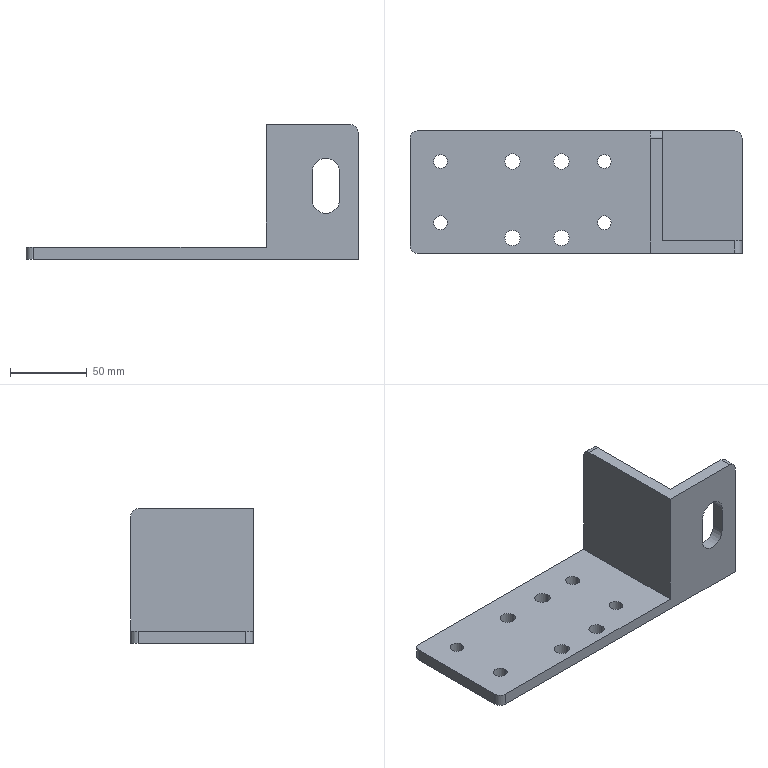Part | SolidWorks | features BaseBody 1 | 1 solid | 37 faces | box 217 x 80 x 88 mm | volume 213969 mm3 | cylinder 24 | plane 13 | commonest cylinder face diameters 10 x13 9 x8 18 x3
STEP:
#1=CARTESIAN_POINT('',(-84.,20.,8.));
#2=VERTEX_POINT('',#1);
#3=CARTESIAN_POINT('',(-93.,20.,8.));
#4=VERTEX_POINT('',#3);
#5=CARTESIAN_POINT('',(-88.5,20.,8.));
#6=DIRECTION('',(0.,0.,-1.));
#7=DIRECTION('',(-1.,0.,0.));
#8=AXIS2_PLACEMENT_3D('',#5,#6,#7);
#9=CIRCLE('',#8,4.5);
#10=EDGE_CURVE('',#2,#4,#9,.T.);
#11=ORIENTED_EDGE('',*,*,#10,.F.);
#12=CARTESIAN_POINT('',(-84.,20.,0.));
#13=VERTEX_POINT('',#12);
#14=CARTESIAN_POINT('',(-84.,20.,10.));
#15=DIRECTION('',(0.,0.,-1.));
#16=VECTOR('',#15,1000.);
#17=LINE('',#14,#16);
#18=EDGE_CURVE('',#2,#13,#17,.T.);
#19=ORIENTED_EDGE('',*,*,#18,.T.);
#20=CARTESIAN_POINT('',(-93.,20.,0.));
#21=VERTEX_POINT('',#20);
#22=CARTESIAN_POINT('',(-88.5,20.,0.));
#23=DIRECTION('',(0.,0.,-1.));
#24=DIRECTION('',(-1.,0.,0.));
#25=AXIS2_PLACEMENT_3D('',#22,#23,#24);
#26=CIRCLE('',#25,4.5);
#27=EDGE_CURVE('',#13,#21,#26,.T.);
#28=ORIENTED_EDGE('',*,*,#27,.T.);
#29=CARTESIAN_POINT('',(-93.,20.,10.));
#30=DIRECTION('',(0.,0.,-1.));
#31=VECTOR('',#30,1000.);
#32=LINE('',#29,#31);
#33=EDGE_CURVE('',#4,#21,#32,.T.);
#34=ORIENTED_EDGE('',*,*,#33,.F.);
#35=EDGE_LOOP('',(#11,#19,#28,#34));
#36=FACE_OUTER_BOUND('',#35,.T.);
#37=CARTESIAN_POINT('',(-88.5,20.,10.));
#38=DIRECTION('',(0.,0.,-1.));
#39=DIRECTION('',(-1.,0.,0.));
#40=AXIS2_PLACEMENT_3D('',#37,#38,#39);
#41=CYLINDRICAL_SURFACE('',#40,4.5);
#42=ADVANCED_FACE('',(#36),#41,.F.);
#43=CARTESIAN_POINT('',(23.,-20.,8.));
#44=VERTEX_POINT('',#43);
#45=CARTESIAN_POINT('',(14.,-20.,8.));
#46=VERTEX_POINT('',#45);
#47=CARTESIAN_POINT('',(18.5,-20.,8.));
#48=DIRECTION('',(0.,0.,-1.));
#49=DIRECTION('',(-1.,0.,0.));
#50=AXIS2_PLACEMENT_3D('',#47,#48,#49);
#51=CIRCLE('',#50,4.5);
#52=EDGE_CURVE('',#44,#46,#51,.T.);
#53=ORIENTED_EDGE('',*,*,#52,.F.);
#54=CARTESIAN_POINT('',(23.,-20.,0.));
#55=VERTEX_POINT('',#54);
#56=CARTESIAN_POINT('',(23.,-20.,10.));
#57=DIRECTION('',(0.,0.,-1.));
#58=VECTOR('',#57,1000.);
#59=LINE('',#56,#58);
#60=EDGE_CURVE('',#44,#55,#59,.T.);
#61=ORIENTED_EDGE('',*,*,#60,.T.);
#62=CARTESIAN_POINT('',(14.,-20.,0.));
#63=VERTEX_POINT('',#62);
#64=CARTESIAN_POINT('',(18.5,-20.,0.));
#65=DIRECTION('',(0.,0.,-1.));
#66=DIRECTION('',(-1.,0.,0.));
#67=AXIS2_PLACEMENT_3D('',#64,#65,#66);
#68=CIRCLE('',#67,4.5);
#69=EDGE_CURVE('',#55,#63,#68,.T.);
#70=ORIENTED_EDGE('',*,*,#69,.T.);
#71=CARTESIAN_POINT('',(14.,-20.,10.));
#72=DIRECTION('',(0.,0.,-1.));
#73=VECTOR('',#72,1000.);
#74=LINE('',#71,#73);
#75=EDGE_CURVE('',#46,#63,#74,.T.);
#76=ORIENTED_EDGE('',*,*,#75,.F.);
#77=EDGE_LOOP('',(#53,#61,#70,#76));
#78=FACE_OUTER_BOUND('',#77,.T.);
#79=CARTESIAN_POINT('',(18.5,-20.,10.));
#80=DIRECTION('',(0.,0.,-1.));
#81=DIRECTION('',(-1.,0.,0.));
#82=AXIS2_PLACEMENT_3D('',#79,#80,#81);
#83=CYLINDRICAL_SURFACE('',#82,4.5);
#84=ADVANCED_FACE('',(#78),#83,.F.);
#85=CARTESIAN_POINT('',(23.,20.,8.));
#86=VERTEX_POINT('',#85);
#87=CARTESIAN_POINT('',(14.,20.,8.));
#88=VERTEX_POINT('',#87);
#89=CARTESIAN_POINT('',(18.5,20.,8.));
#90=DIRECTION('',(0.,0.,-1.));
#91=DIRECTION('',(-1.,0.,0.));
#92=AXIS2_PLACEMENT_3D('',#89,#90,#91);
#93=CIRCLE('',#92,4.5);
#94=EDGE_CURVE('',#86,#88,#93,.T.);
#95=ORIENTED_EDGE('',*,*,#94,.F.);
#96=CARTESIAN_POINT('',(23.,20.,0.));
#97=VERTEX_POINT('',#96);
#98=CARTESIAN_POINT('',(23.,20.,10.));
#99=DIRECTION('',(0.,0.,-1.));
#100=VECTOR('',#99,1000.);
#101=LINE('',#98,#100);
#102=EDGE_CURVE('',#86,#97,#101,.T.);
#103=ORIENTED_EDGE('',*,*,#102,.T.);
#104=CARTESIAN_POINT('',(14.,20.,0.));
#105=VERTEX_POINT('',#104);
#106=CARTESIAN_POINT('',(18.5,20.,0.));
#107=DIRECTION('',(0.,0.,-1.));
#108=DIRECTION('',(-1.,0.,0.));
#109=AXIS2_PLACEMENT_3D('',#106,#107,#108);
#110=CIRCLE('',#109,4.5);
#111=EDGE_CURVE('',#97,#105,#110,.T.);
#112=ORIENTED_EDGE('',*,*,#111,.T.);
#113=CARTESIAN_POINT('',(14.,20.,10.));
#114=DIRECTION('',(0.,0.,-1.));
#115=VECTOR('',#114,1000.);
#116=LINE('',#113,#115);
#117=EDGE_CURVE('',#88,#105,#116,.T.);
#118=ORIENTED_EDGE('',*,*,#117,.F.);
#119=EDGE_LOOP('',(#95,#103,#112,#118));
#120=FACE_OUTER_BOUND('',#119,.T.);
#121=CARTESIAN_POINT('',(18.5,20.,10.));
#122=DIRECTION('',(0.,0.,-1.));
#123=DIRECTION('',(-1.,0.,0.));
#124=AXIS2_PLACEMENT_3D('',#121,#122,#123);
#125=CYLINDRICAL_SURFACE('',#124,4.5);
#126=ADVANCED_FACE('',(#120),#125,.F.);
#127=CARTESIAN_POINT('',(-84.,-20.,8.));
#128=VERTEX_POINT('',#127);
#129=CARTESIAN_POINT('',(-93.,-20.,8.));
#130=VERTEX_POINT('',#129);
#131=CARTESIAN_POINT('',(-88.5,-20.,8.));
#132=DIRECTION('',(0.,0.,-1.));
#133=DIRECTION('',(-1.,0.,0.));
#134=AXIS2_PLACEMENT_3D('',#131,#132,#133);
#135=CIRCLE('',#134,4.5);
#136=EDGE_CURVE('',#128,#130,#135,.T.);
#137=ORIENTED_EDGE('',*,*,#136,.F.);
#138=CARTESIAN_POINT('',(-84.,-20.,0.));
#139=VERTEX_POINT('',#138);
#140=CARTESIAN_POINT('',(-84.,-20.,10.));
#141=DIRECTION('',(0.,0.,-1.));
#142=VECTOR('',#141,1000.);
#143=LINE('',#140,#142);
#144=EDGE_CURVE('',#128,#139,#143,.T.);
#145=ORIENTED_EDGE('',*,*,#144,.T.);
#146=CARTESIAN_POINT('',(-93.,-20.,0.));
#147=VERTEX_POINT('',#146);
#148=CARTESIAN_POINT('',(-88.5,-20.,0.));
#149=DIRECTION('',(0.,0.,-1.));
#150=DIRECTION('',(-1.,0.,0.));
#151=AXIS2_PLACEMENT_3D('',#148,#149,#150);
#152=CIRCLE('',#151,4.5);
#153=EDGE_CURVE('',#139,#147,#152,.T.);
#154=ORIENTED_EDGE('',*,*,#153,.T.);
#155=CARTESIAN_POINT('',(-93.,-20.,10.));
#156=DIRECTION('',(0.,0.,-1.));
#157=VECTOR('',#156,1000.);
#158=LINE('',#155,#157);
#159=EDGE_CURVE('',#130,#147,#158,.T.);
#160=ORIENTED_EDGE('',*,*,#159,.F.);
#161=EDGE_LOOP('',(#137,#145,#154,#160));
#162=FACE_OUTER_BOUND('',#161,.T.);
#163=CARTESIAN_POINT('',(-88.5,-20.,10.));
#164=DIRECTION('',(0.,0.,-1.));
#165=DIRECTION('',(-1.,0.,0.));
#166=AXIS2_PLACEMENT_3D('',#163,#164,#165);
#167=CYLINDRICAL_SURFACE('',#166,4.5);
#168=ADVANCED_FACE('',(#162),#167,.F.);
#169=CARTESIAN_POINT('',(87.5,-40.,66.));
#170=VERTEX_POINT('',#169);
#171=CARTESIAN_POINT('',(96.5,-40.,57.));
#172=VERTEX_POINT('',#171);
#173=CARTESIAN_POINT('',(87.5,-40.,57.));
#174=DIRECTION('',(0.,1.,0.));
#175=DIRECTION('',(0.,0.,1.));
#176=AXIS2_PLACEMENT_3D('',#173,#174,#175);
#177=CIRCLE('',#176,9.);
#178=EDGE_CURVE('',#170,#172,#177,.T.);
#179=ORIENTED_EDGE('',*,*,#178,.F.);
#180=CARTESIAN_POINT('',(87.5,-32.,66.));
#181=VERTEX_POINT('',#180);
#182=CARTESIAN_POINT('',(87.5,-142.,66.));
#183=DIRECTION('',(0.,1.,0.));
#184=VECTOR('',#183,1000.);
#185=LINE('',#182,#184);
#186=EDGE_CURVE('',#170,#181,#185,.T.);
#187=ORIENTED_EDGE('',*,*,#186,.T.);
#188=CARTESIAN_POINT('',(96.5,-32.,57.));
#189=VERTEX_POINT('',#188);
#190=CARTESIAN_POINT('',(87.5,-32.,57.));
#191=DIRECTION('',(0.,1.,0.));
#192=DIRECTION('',(0.,0.,1.));
#193=AXIS2_PLACEMENT_3D('',#190,#191,#192);
#194=CIRCLE('',#193,9.);
#195=EDGE_CURVE('',#181,#189,#194,.T.);
#196=ORIENTED_EDGE('',*,*,#195,.T.);
#197=CARTESIAN_POINT('',(96.5,-142.,57.));
#198=DIRECTION('',(0.,1.,0.));
#199=VECTOR('',#198,1000.);
#200=LINE('',#197,#199);
#201=EDGE_CURVE('',#172,#189,#200,.T.);
#202=ORIENTED_EDGE('',*,*,#201,.F.);
#203=EDGE_LOOP('',(#179,#187,#196,#202));
#204=FACE_OUTER_BOUND('',#203,.T.);
#205=CARTESIAN_POINT('',(87.5,-142.,57.));
#206=DIRECTION('',(0.,1.,0.));
#207=DIRECTION('',(0.,0.,1.));
#208=AXIS2_PLACEMENT_3D('',#205,#206,#207);
#209=CYLINDRICAL_SURFACE('',#208,9.);
#210=ADVANCED_FACE('',(#204),#209,.F.);
#211=CARTESIAN_POINT('',(-4.5,20.,0.));
#212=VERTEX_POINT('',#211);
#213=CARTESIAN_POINT('',(-14.5,20.,0.));
#214=VERTEX_POINT('',#213);
#215=CARTESIAN_POINT('',(-9.5,20.,0.));
#216=DIRECTION('',(0.,0.,-1.));
#217=DIRECTION('',(-1.,0.,0.));
#218=AXIS2_PLACEMENT_3D('',#215,#216,#217);
#219=CIRCLE('',#218,5.);
#220=EDGE_CURVE('',#212,#214,#219,.T.);
#221=ORIENTED_EDGE('',*,*,#220,.T.);
#222=CARTESIAN_POINT('',(-14.5,20.,8.));
#223=VERTEX_POINT('',#222);
#224=CARTESIAN_POINT('',(-14.5,20.,-2.));
#225=DIRECTION('',(0.,0.,1.));
#226=VECTOR('',#225,1000.);
#227=LINE('',#224,#226);
#228=EDGE_CURVE('',#214,#223,#227,.T.);
#229=ORIENTED_EDGE('',*,*,#228,.T.);
#230=CARTESIAN_POINT('',(-4.5,20.,8.));
#231=VERTEX_POINT('',#230);
#232=CARTESIAN_POINT('',(-9.5,20.,8.));
#233=DIRECTION('',(0.,0.,1.));
#234=DIRECTION('',(1.,0.,0.));
#235=AXIS2_PLACEMENT_3D('',#232,#233,#234);
#236=CIRCLE('',#235,5.);
#237=EDGE_CURVE('',#223,#231,#236,.T.);
#238=ORIENTED_EDGE('',*,*,#237,.T.);
#239=CARTESIAN_POINT('',(-4.5,20.,-2.));
#240=DIRECTION('',(0.,0.,1.));
#241=VECTOR('',#240,1000.);
#242=LINE('',#239,#241);
#243=EDGE_CURVE('',#212,#231,#242,.T.);
#244=ORIENTED_EDGE('',*,*,#243,.F.);
#245=EDGE_LOOP('',(#221,#229,#238,#244));
#246=FACE_OUTER_BOUND('',#245,.T.);
#247=CARTESIAN_POINT('',(-9.5,20.,-2.));
#248=DIRECTION('',(0.,0.,1.));
#249=DIRECTION('',(1.,0.,0.));
#250=AXIS2_PLACEMENT_3D('',#247,#248,#249);
#251=CYLINDRICAL_SURFACE('',#250,5.);
#252=ADVANCED_FACE('',(#246),#251,.F.);
#253=CARTESIAN_POINT('',(-36.5,-30.,0.));
#254=VERTEX_POINT('',#253);
#255=CARTESIAN_POINT('',(-46.5,-30.,0.));
#256=VERTEX_POINT('',#255);
#257=CARTESIAN_POINT('',(-41.5,-30.,0.));
#258=DIRECTION('',(0.,0.,-1.));
#259=DIRECTION('',(-1.,0.,0.));
#260=AXIS2_PLACEMENT_3D('',#257,#258,#259);
#261=CIRCLE('',#260,5.);
#262=EDGE_CURVE('',#254,#256,#261,.T.);
#263=ORIENTED_EDGE('',*,*,#262,.T.);
#264=CARTESIAN_POINT('',(-46.5,-30.,8.));
#265=VERTEX_POINT('',#264);
#266=CARTESIAN_POINT('',(-46.5,-30.,-2.));
#267=DIRECTION('',(0.,0.,1.));
#268=VECTOR('',#267,1000.);
#269=LINE('',#266,#268);
#270=EDGE_CURVE('',#256,#265,#269,.T.);
#271=ORIENTED_EDGE('',*,*,#270,.T.);
#272=CARTESIAN_POINT('',(-36.5,-30.,8.));
#273=VERTEX_POINT('',#272);
#274=CARTESIAN_POINT('',(-41.5,-30.,8.));
#275=DIRECTION('',(0.,0.,1.));
#276=DIRECTION('',(1.,0.,0.));
#277=AXIS2_PLACEMENT_3D('',#274,#275,#276);
#278=CIRCLE('',#277,5.);
#279=EDGE_CURVE('',#265,#273,#278,.T.);
#280=ORIENTED_EDGE('',*,*,#279,.T.);
#281=CARTESIAN_POINT('',(-36.5,-30.,-2.));
#282=DIRECTION('',(0.,0.,1.));
#283=VECTOR('',#282,1000.);
#284=LINE('',#281,#283);
#285=EDGE_CURVE('',#254,#273,#284,.T.);
#286=ORIENTED_EDGE('',*,*,#285,.F.);
#287=EDGE_LOOP('',(#263,#271,#280,#286));
#288=FACE_OUTER_BOUND('',#287,.T.);
#289=CARTESIAN_POINT('',(-41.5,-30.,-2.));
#290=DIRECTION('',(0.,0.,1.));
#291=DIRECTION('',(1.,0.,0.));
#292=AXIS2_PLACEMENT_3D('',#289,#290,#291);
#293=CYLINDRICAL_SURFACE('',#292,5.);
#294=ADVANCED_FACE('',(#288),#293,.F.);
#295=CARTESIAN_POINT('',(-36.5,20.,0.));
#296=VERTEX_POINT('',#295);
#297=CARTESIAN_POINT('',(-46.5,20.,0.));
#298=VERTEX_POINT('',#297);
#299=CARTESIAN_POINT('',(-41.5,20.,0.));
#300=DIRECTION('',(0.,0.,-1.));
#301=DIRECTION('',(-1.,0.,0.));
#302=AXIS2_PLACEMENT_3D('',#299,#300,#301);
#303=CIRCLE('',#302,5.);
#304=EDGE_CURVE('',#296,#298,#303,.T.);
#305=ORIENTED_EDGE('',*,*,#304,.T.);
#306=CARTESIAN_POINT('',(-46.5,20.,8.));
#307=VERTEX_POINT('',#306);
#308=CARTESIAN_POINT('',(-46.5,20.,-2.));
#309=DIRECTION('',(0.,0.,1.));
#310=VECTOR('',#309,1000.);
#311=LINE('',#308,#310);
#312=EDGE_CURVE('',#298,#307,#311,.T.);
#313=ORIENTED_EDGE('',*,*,#312,.T.);
#314=CARTESIAN_POINT('',(-36.5,20.,8.));
#315=VERTEX_POINT('',#314);
#316=CARTESIAN_POINT('',(-41.5,20.,8.));
#317=DIRECTION('',(0.,0.,1.));
#318=DIRECTION('',(1.,0.,0.));
#319=AXIS2_PLACEMENT_3D('',#316,#317,#318);
#320=CIRCLE('',#319,5.);
#321=EDGE_CURVE('',#307,#315,#320,.T.);
#322=ORIENTED_EDGE('',*,*,#321,.T.);
#323=CARTESIAN_POINT('',(-36.5,20.,-2.));
#324=DIRECTION('',(0.,0.,1.));
#325=VECTOR('',#324,1000.);
#326=LINE('',#323,#325);
#327=EDGE_CURVE('',#296,#315,#326,.T.);
#328=ORIENTED_EDGE('',*,*,#327,.F.);
#329=EDGE_LOOP('',(#305,#313,#322,#328));
#330=FACE_OUTER_BOUND('',#329,.T.);
#331=CARTESIAN_POINT('',(-41.5,20.,-2.));
#332=DIRECTION('',(0.,0.,1.));
#333=DIRECTION('',(1.,0.,0.));
#334=AXIS2_PLACEMENT_3D('',#331,#332,#333);
#335=CYLINDRICAL_SURFACE('',#334,5.);
#336=ADVANCED_FACE('',(#330),#335,.F.);
#337=CARTESIAN_POINT('',(-4.5,-30.,0.));
#338=VERTEX_POINT('',#337);
#339=CARTESIAN_POINT('',(-14.5,-30.,0.));
#340=VERTEX_POINT('',#339);
#341=CARTESIAN_POINT('',(-9.5,-30.,0.));
#342=DIRECTION('',(0.,0.,-1.));
#343=DIRECTION('',(-1.,0.,0.));
#344=AXIS2_PLACEMENT_3D('',#341,#342,#343);
#345=CIRCLE('',#344,5.);
#346=EDGE_CURVE('',#338,#340,#345,.T.);
#347=ORIENTED_EDGE('',*,*,#346,.T.);
#348=CARTESIAN_POINT('',(-14.5,-30.,8.));
#349=VERTEX_POINT('',#348);
#350=CARTESIAN_POINT('',(-14.5,-30.,-2.));
#351=DIRECTION('',(0.,0.,1.));
#352=VECTOR('',#351,1000.);
#353=LINE('',#350,#352);
#354=EDGE_CURVE('',#340,#349,#353,.T.);
#355=ORIENTED_EDGE('',*,*,#354,.T.);
#356=CARTESIAN_POINT('',(-4.5,-30.,8.));
#357=VERTEX_POINT('',#356);
#358=CARTESIAN_POINT('',(-9.5,-30.,8.));
#359=DIRECTION('',(0.,0.,1.));
#360=DIRECTION('',(1.,0.,0.));
#361=AXIS2_PLACEMENT_3D('',#358,#359,#360);
#362=CIRCLE('',#361,5.);
#363=EDGE_CURVE('',#349,#357,#362,.T.);
#364=ORIENTED_EDGE('',*,*,#363,.T.);
#365=CARTESIAN_POINT('',(-4.5,-30.,-2.));
#366=DIRECTION('',(0.,0.,1.));
#367=VECTOR('',#366,1000.);
#368=LINE('',#365,#367);
#369=EDGE_CURVE('',#338,#357,#368,.T.);
#370=ORIENTED_EDGE('',*,*,#369,.F.);
#371=EDGE_LOOP('',(#347,#355,#364,#370));
#372=FACE_OUTER_BOUND('',#371,.T.);
#373=CARTESIAN_POINT('',(-9.5,-30.,-2.));
#374=DIRECTION('',(0.,0.,1.));
#375=DIRECTION('',(1.,0.,0.));
#376=AXIS2_PLACEMENT_3D('',#373,#374,#375);
#377=CYLINDRICAL_SURFACE('',#376,5.);
#378=ADVANCED_FACE('',(#372),#377,.F.);
#379=CARTESIAN_POINT('',(-88.5,20.,8.));
#380=DIRECTION('',(0.,0.,-1.));
#381=DIRECTION('',(-1.,0.,0.));
#382=AXIS2_PLACEMENT_3D('',#379,#380,#381);
#383=CIRCLE('',#382,4.5);
#384=EDGE_CURVE('',#4,#2,#383,.T.);
#385=ORIENTED_EDGE('',*,*,#384,.T.);
#386=ORIENTED_EDGE('',*,*,#10,.T.);
#387=EDGE_LOOP('',(#385,#386));
#388=FACE_BOUND('',#387,.T.);
#389=CARTESIAN_POINT('',(18.5,-20.,8.));
#390=DIRECTION('',(0.,0.,-1.));
#391=DIRECTION('',(-1.,0.,0.));
#392=AXIS2_PLACEMENT_3D('',#389,#390,#391);
#393=CIRCLE('',#392,4.5);
#394=EDGE_CURVE('',#46,#44,#393,.T.);
#395=ORIENTED_EDGE('',*,*,#394,.T.);
#396=ORIENTED_EDGE('',*,*,#52,.T.);
#397=EDGE_LOOP('',(#395,#396));
#398=FACE_BOUND('',#397,.T.);
#399=CARTESIAN_POINT('',(18.5,20.,8.));
#400=DIRECTION('',(0.,0.,-1.));
#401=DIRECTION('',(-1.,0.,0.));
#402=AXIS2_PLACEMENT_3D('',#399,#400,#401);
#403=CIRCLE('',#402,4.5);
#404=EDGE_CURVE('',#88,#86,#403,.T.);
#405=ORIENTED_EDGE('',*,*,#404,.T.);
#406=ORIENTED_EDGE('',*,*,#94,.T.);
#407=EDGE_LOOP('',(#405,#406));
#408=FACE_BOUND('',#407,.T.);
#409=CARTESIAN_POINT('',(-88.5,-20.,8.));
#410=DIRECTION('',(0.,0.,-1.));
#411=DIRECTION('',(-1.,0.,0.));
#412=AXIS2_PLACEMENT_3D('',#409,#410,#411);
#413=CIRCLE('',#412,4.5);
#414=EDGE_CURVE('',#130,#128,#413,.T.);
#415=ORIENTED_EDGE('',*,*,#414,.T.);
#416=ORIENTED_EDGE('',*,*,#136,.T.);
#417=EDGE_LOOP('',(#415,#416));
#418=FACE_BOUND('',#417,.T.);
#419=CARTESIAN_POINT('',(-9.5,-30.,8.));
#420=DIRECTION('',(0.,0.,1.));
#421=DIRECTION('',(1.,0.,0.));
#422=AXIS2_PLACEMENT_3D('',#419,#420,#421);
#423=CIRCLE('',#422,5.);
#424=EDGE_CURVE('',#357,#349,#423,.T.);
#425=ORIENTED_EDGE('',*,*,#424,.F.);
#426=ORIENTED_EDGE('',*,*,#363,.F.);
#427=EDGE_LOOP('',(#425,#426));
#428=FACE_BOUND('',#427,.T.);
#429=CARTESIAN_POINT('',(-41.5,20.,8.));
#430=DIRECTION('',(0.,0.,1.));
#431=DIRECTION('',(1.,0.,0.));
#432=AXIS2_PLACEMENT_3D('',#429,#430,#431);
#433=CIRCLE('',#432,5.);
#434=EDGE_CURVE('',#315,#307,#433,.T.);
#435=ORIENTED_EDGE('',*,*,#434,.F.);
#436=ORIENTED_EDGE('',*,*,#321,.F.);
#437=EDGE_LOOP('',(#435,#436));
#438=FACE_BOUND('',#437,.T.);
#439=CARTESIAN_POINT('',(-41.5,-30.,8.));
#440=DIRECTION('',(0.,0.,1.));
#441=DIRECTION('',(1.,0.,0.));
#442=AXIS2_PLACEMENT_3D('',#439,#440,#441);
#443=CIRCLE('',#442,5.);
#444=EDGE_CURVE('',#273,#265,#443,.T.);
#445=ORIENTED_EDGE('',*,*,#444,.F.);
#446=ORIENTED_EDGE('',*,*,#279,.F.);
#447=EDGE_LOOP('',(#445,#446));
#448=FACE_BOUND('',#447,.T.);
#449=CARTESIAN_POINT('',(-9.5,20.,8.));
#450=DIRECTION('',(0.,0.,1.));
#451=DIRECTION('',(1.,0.,0.));
#452=AXIS2_PLACEMENT_3D('',#449,#450,#451);
#453=CIRCLE('',#452,5.);
#454=EDGE_CURVE('',#231,#223,#453,.T.);
#455=ORIENTED_EDGE('',*,*,#454,.F.);
#456=ORIENTED_EDGE('',*,*,#237,.F.);
#457=EDGE_LOOP('',(#455,#456));
#458=FACE_BOUND('',#457,.T.);
#459=CARTESIAN_POINT('',(-108.5,35.,8.));
#460=VERTEX_POINT('',#459);
#461=CARTESIAN_POINT('',(-108.5,-35.,8.));
#462=VERTEX_POINT('',#461);
#463=CARTESIAN_POINT('',(-108.5,-40.,8.));
#464=DIRECTION('',(0.,-1.,0.));
#465=VECTOR('',#464,1000.);
#466=LINE('',#463,#465);
#467=EDGE_CURVE('',#460,#462,#466,.T.);
#468=ORIENTED_EDGE('',*,*,#467,.T.);
#469=CARTESIAN_POINT('',(-103.5,-40.,8.));
#470=VERTEX_POINT('',#469);
#471=CARTESIAN_POINT('',(-103.5,-35.,8.));
#472=DIRECTION('',(0.,0.,1.));
#473=DIRECTION('',(-1.,0.,0.));
#474=AXIS2_PLACEMENT_3D('',#471,#472,#473);
#475=CIRCLE('',#474,5.);
#476=EDGE_CURVE('',#462,#470,#475,.T.);
#477=ORIENTED_EDGE('',*,*,#476,.T.);
#478=CARTESIAN_POINT('',(48.5,-40.,8.));
#479=VERTEX_POINT('',#478);
#480=CARTESIAN_POINT('',(-108.5,-40.,8.));
#481=DIRECTION('',(1.,0.,0.));
#482=VECTOR('',#481,1000.);
#483=LINE('',#480,#482);
#484=EDGE_CURVE('',#470,#479,#483,.T.);
#485=ORIENTED_EDGE('',*,*,#484,.T.);
#486=CARTESIAN_POINT('',(48.5,40.,8.));
#487=VERTEX_POINT('',#486);
#488=CARTESIAN_POINT('',(48.5,-40.,8.));
#489=DIRECTION('',(0.,-1.,0.));
#490=VECTOR('',#489,1000.);
#491=LINE('',#488,#490);
#492=EDGE_CURVE('',#487,#479,#491,.T.);
#493=ORIENTED_EDGE('',*,*,#492,.F.);
#494=CARTESIAN_POINT('',(-103.5,40.,8.));
#495=VERTEX_POINT('',#494);
#496=CARTESIAN_POINT('',(-108.5,40.,8.));
#497=DIRECTION('',(-1.,0.,0.));
#498=VECTOR('',#497,1000.);
#499=LINE('',#496,#498);
#500=EDGE_CURVE('',#487,#495,#499,.T.);
#501=ORIENTED_EDGE('',*,*,#500,.T.);
#502=CARTESIAN_POINT('',(-103.5,35.,8.));
#503=DIRECTION('',(0.,0.,1.));
#504=DIRECTION('',(-1.,0.,0.));
#505=AXIS2_PLACEMENT_3D('',#502,#503,#504);
#506=CIRCLE('',#505,5.);
#507=EDGE_CURVE('',#495,#460,#506,.T.);
#508=ORIENTED_EDGE('',*,*,#507,.T.);
#509=EDGE_LOOP('',(#468,#477,#485,#493,#501,#508));
#510=FACE_OUTER_BOUND('',#509,.T.);
#511=CARTESIAN_POINT('',(0.,0.,8.));
#512=DIRECTION('',(0.,0.,-1.));
#513=DIRECTION('',(-1.,0.,0.));
#514=AXIS2_PLACEMENT_3D('',#511,#512,#513);
#515=PLANE('',#514);
#516=ADVANCED_FACE('',(#388,#398,#408,#418,#428,#438,#448,#458,#510),#515,.F.);
#517=CARTESIAN_POINT('',(108.5,-32.,8.));
#518=VERTEX_POINT('',#517);
#519=CARTESIAN_POINT('',(108.5,35.,8.));
#520=VERTEX_POINT('',#519);
#521=CARTESIAN_POINT('',(108.5,-40.,8.));
#522=DIRECTION('',(0.,1.,0.));
#523=VECTOR('',#522,1000.);
#524=LINE('',#521,#523);
#525=EDGE_CURVE('',#518,#520,#524,.T.);
#526=ORIENTED_EDGE('',*,*,#525,.T.);
#527=CARTESIAN_POINT('',(103.5,40.,8.));
#528=VERTEX_POINT('',#527);
#529=CARTESIAN_POINT('',(103.5,35.,8.));
#530=DIRECTION('',(0.,0.,1.));
#531=DIRECTION('',(-1.,0.,0.));
#532=AXIS2_PLACEMENT_3D('',#529,#530,#531);
#533=CIRCLE('',#532,5.);
#534=EDGE_CURVE('',#520,#528,#533,.T.);
#535=ORIENTED_EDGE('',*,*,#534,.T.);
#536=CARTESIAN_POINT('',(56.5,40.,8.));
#537=VERTEX_POINT('',#536);
#538=CARTESIAN_POINT('',(-108.5,40.,8.));
#539=DIRECTION('',(-1.,0.,0.));
#540=VECTOR('',#539,1000.);
#541=LINE('',#538,#540);
#542=EDGE_CURVE('',#528,#537,#541,.T.);
#543=ORIENTED_EDGE('',*,*,#542,.T.);
#544=CARTESIAN_POINT('',(56.5,-32.,8.));
#545=VERTEX_POINT('',#544);
#546=CARTESIAN_POINT('',(56.5,40.,8.));
#547=DIRECTION('',(0.,1.,0.));
#548=VECTOR('',#547,1000.);
#549=LINE('',#546,#548);
#550=EDGE_CURVE('',#545,#537,#549,.T.);
#551=ORIENTED_EDGE('',*,*,#550,.F.);
#552=CARTESIAN_POINT('',(56.5,-32.,8.));
#553=DIRECTION('',(-1.,0.,0.));
#554=VECTOR('',#553,1000.);
#555=LINE('',#552,#554);
#556=EDGE_CURVE('',#518,#545,#555,.T.);
#557=ORIENTED_EDGE('',*,*,#556,.F.);
#558=EDGE_LOOP('',(#526,#535,#543,#551,#557));
#559=FACE_OUTER_BOUND('',#558,.T.);
#560=CARTESIAN_POINT('',(0.,0.,8.));
#561=DIRECTION('',(0.,0.,-1.));
#562=DIRECTION('',(-1.,0.,0.));
#563=AXIS2_PLACEMENT_3D('',#560,#561,#562);
#564=PLANE('',#563);
#565=ADVANCED_FACE('',(#559),#564,.F.);
#566=CARTESIAN_POINT('',(108.5,-40.,0.));
#567=VERTEX_POINT('',#566);
#568=CARTESIAN_POINT('',(108.5,35.,0.));
#569=VERTEX_POINT('',#568);
#570=CARTESIAN_POINT('',(108.5,-40.,0.));
#571=DIRECTION('',(0.,1.,0.));
#572=VECTOR('',#571,1000.);
#573=LINE('',#570,#572);
#574=EDGE_CURVE('',#567,#569,#573,.T.);
#575=ORIENTED_EDGE('',*,*,#574,.T.);
#576=CARTESIAN_POINT('',(108.5,35.,8.));
#577=DIRECTION('',(0.,0.,1.));
#578=VECTOR('',#577,1000.);
#579=LINE('',#576,#578);
#580=EDGE_CURVE('',#569,#520,#579,.T.);
#581=ORIENTED_EDGE('',*,*,#580,.T.);
#582=ORIENTED_EDGE('',*,*,#525,.F.);
#583=CARTESIAN_POINT('',(108.5,-32.,83.));
#584=VERTEX_POINT('',#583);
#585=CARTESIAN_POINT('',(108.5,-32.,88.));
#586=DIRECTION('',(0.,0.,-1.));
#587=VECTOR('',#586,1000.);
#588=LINE('',#585,#587);
#589=EDGE_CURVE('',#584,#518,#588,.T.);
#590=ORIENTED_EDGE('',*,*,#589,.F.);
#591=CARTESIAN_POINT('',(108.5,-40.,83.));
#592=VERTEX_POINT('',#591);
#593=CARTESIAN_POINT('',(108.5,-40.,83.));
#594=DIRECTION('',(0.,-1.,0.));
#595=VECTOR('',#594,1000.);
#596=LINE('',#593,#595);
#597=EDGE_CURVE('',#584,#592,#596,.T.);
#598=ORIENTED_EDGE('',*,*,#597,.T.);
#599=CARTESIAN_POINT('',(108.5,-40.,8.));
#600=DIRECTION('',(0.,0.,-1.));
#601=VECTOR('',#600,1000.);
#602=LINE('',#599,#601);
#603=EDGE_CURVE('',#592,#567,#602,.T.);
#604=ORIENTED_EDGE('',*,*,#603,.T.);
#605=EDGE_LOOP('',(#575,#581,#582,#590,#598,#604));
#606=FACE_OUTER_BOUND('',#605,.T.);
#607=CARTESIAN_POINT('',(108.5,-40.,8.));
#608=DIRECTION('',(-1.,0.,0.));
#609=DIRECTION('',(0.,0.,1.));
#610=AXIS2_PLACEMENT_3D('',#607,#608,#609);
#611=PLANE('',#610);
#612=ADVANCED_FACE('',(#606),#611,.F.);
#613=CARTESIAN_POINT('',(48.5,40.,83.));
#614=VERTEX_POINT('',#613);
#615=CARTESIAN_POINT('',(48.5,40.,88.));
#616=DIRECTION('',(0.,0.,-1.));
#617=VECTOR('',#616,1000.);
#618=LINE('',#615,#617);
#619=EDGE_CURVE('',#614,#487,#618,.T.);
#620=ORIENTED_EDGE('',*,*,#619,.F.);
#621=CARTESIAN_POINT('',(56.5,40.,83.));
#622=VERTEX_POINT('',#621);
#623=CARTESIAN_POINT('',(-108.5,40.,83.));
#624=DIRECTION('',(1.,0.,0.));
#625=VECTOR('',#624,1000.);
#626=LINE('',#623,#625);
#627=EDGE_CURVE('',#614,#622,#626,.T.);
#628=ORIENTED_EDGE('',*,*,#627,.T.);
#629=CARTESIAN_POINT('',(56.5,40.,88.));
#630=DIRECTION('',(0.,0.,-1.));
#631=VECTOR('',#630,1000.);
#632=LINE('',#629,#631);
#633=EDGE_CURVE('',#622,#537,#632,.T.);
#634=ORIENTED_EDGE('',*,*,#633,.T.);
#635=ORIENTED_EDGE('',*,*,#542,.F.);
#636=CARTESIAN_POINT('',(103.5,40.,0.));
#637=VERTEX_POINT('',#636);
#638=CARTESIAN_POINT('',(103.5,40.,8.));
#639=DIRECTION('',(0.,0.,-1.));
#640=VECTOR('',#639,1000.);
#641=LINE('',#638,#640);
#642=EDGE_CURVE('',#528,#637,#641,.T.);
#643=ORIENTED_EDGE('',*,*,#642,.T.);
#644=CARTESIAN_POINT('',(-103.5,40.,0.));
#645=VERTEX_POINT('',#644);
#646=CARTESIAN_POINT('',(-108.5,40.,0.));
#647=DIRECTION('',(-1.,0.,0.));
#648=VECTOR('',#647,1000.);
#649=LINE('',#646,#648);
#650=EDGE_CURVE('',#637,#645,#649,.T.);
#651=ORIENTED_EDGE('',*,*,#650,.T.);
#652=CARTESIAN_POINT('',(-103.5,40.,8.));
#653=DIRECTION('',(0.,0.,1.));
#654=VECTOR('',#653,1000.);
#655=LINE('',#652,#654);
#656=EDGE_CURVE('',#645,#495,#655,.T.);
#657=ORIENTED_EDGE('',*,*,#656,.T.);
#658=ORIENTED_EDGE('',*,*,#500,.F.);
#659=EDGE_LOOP('',(#620,#628,#634,#635,#643,#651,#657,#658));
#660=FACE_OUTER_BOUND('',#659,.T.);
#661=CARTESIAN_POINT('',(-108.5,40.,8.));
#662=DIRECTION('',(0.,-1.,0.));
#663=DIRECTION('',(0.,0.,-1.));
#664=AXIS2_PLACEMENT_3D('',#661,#662,#663);
#665=PLANE('',#664);
#666=ADVANCED_FACE('',(#660),#665,.F.);
#667=CARTESIAN_POINT('',(-108.5,35.,0.));
#668=VERTEX_POINT('',#667);
#669=CARTESIAN_POINT('',(-108.5,-35.,0.));
#670=VERTEX_POINT('',#669);
#671=CARTESIAN_POINT('',(-108.5,-40.,0.));
#672=DIRECTION('',(0.,-1.,0.));
#673=VECTOR('',#672,1000.);
#674=LINE('',#671,#673);
#675=EDGE_CURVE('',#668,#670,#674,.T.);
#676=ORIENTED_EDGE('',*,*,#675,.T.);
#677=CARTESIAN_POINT('',(-108.5,-35.,8.));
#678=DIRECTION('',(0.,0.,1.));
#679=VECTOR('',#678,1000.);
#680=LINE('',#677,#679);
#681=EDGE_CURVE('',#670,#462,#680,.T.);
#682=ORIENTED_EDGE('',*,*,#681,.T.);
#683=ORIENTED_EDGE('',*,*,#467,.F.);
#684=CARTESIAN_POINT('',(-108.5,35.,8.));
#685=DIRECTION('',(0.,0.,-1.));
#686=VECTOR('',#685,1000.);
#687=LINE('',#684,#686);
#688=EDGE_CURVE('',#460,#668,#687,.T.);
#689=ORIENTED_EDGE('',*,*,#688,.T.);
#690=EDGE_LOOP('',(#676,#682,#683,#689));
#691=FACE_OUTER_BOUND('',#690,.T.);
#692=CARTESIAN_POINT('',(-108.5,-40.,8.));
#693=DIRECTION('',(1.,0.,0.));
#694=DIRECTION('',(0.,0.,-1.));
#695=AXIS2_PLACEMENT_3D('',#692,#693,#694);
#696=PLANE('',#695);
#697=ADVANCED_FACE('',(#691),#696,.F.);
#698=CARTESIAN_POINT('',(96.5,-40.,39.));
#699=VERTEX_POINT('',#698);
#700=CARTESIAN_POINT('',(96.5,-40.,8.));
#701=DIRECTION('',(0.,0.,-1.));
#702=VECTOR('',#701,1000.);
#703=LINE('',#700,#702);
#704=EDGE_CURVE('',#172,#699,#703,.T.);
#705=ORIENTED_EDGE('',*,*,#704,.T.);
#706=CARTESIAN_POINT('',(78.5,-40.,39.));
#707=VERTEX_POINT('',#706);
#708=CARTESIAN_POINT('',(87.5,-40.,39.));
#709=DIRECTION('',(0.,1.,0.));
#710=DIRECTION('',(0.,0.,1.));
#711=AXIS2_PLACEMENT_3D('',#708,#709,#710);
#712=CIRCLE('',#711,9.);
#713=EDGE_CURVE('',#699,#707,#712,.T.);
#714=ORIENTED_EDGE('',*,*,#713,.T.);
#715=CARTESIAN_POINT('',(78.5,-40.,57.));
#716=VERTEX_POINT('',#715);
#717=CARTESIAN_POINT('',(78.5,-40.,8.));
#718=DIRECTION('',(0.,0.,1.));
#719=VECTOR('',#718,1000.);
#720=LINE('',#717,#719);
#721=EDGE_CURVE('',#707,#716,#720,.T.);
#722=ORIENTED_EDGE('',*,*,#721,.T.);
#723=CARTESIAN_POINT('',(87.5,-40.,57.));
#724=DIRECTION('',(0.,1.,0.));
#725=DIRECTION('',(0.,0.,1.));
#726=AXIS2_PLACEMENT_3D('',#723,#724,#725);
#727=CIRCLE('',#726,9.);
#728=EDGE_CURVE('',#716,#170,#727,.T.);
#729=ORIENTED_EDGE('',*,*,#728,.T.);
#730=ORIENTED_EDGE('',*,*,#178,.T.);
#731=EDGE_LOOP('',(#705,#714,#722,#729,#730));
#732=FACE_BOUND('',#731,.T.);
#733=ORIENTED_EDGE('',*,*,#603,.F.);
#734=CARTESIAN_POINT('',(103.5,-40.,88.));
#735=VERTEX_POINT('',#734);
#736=CARTESIAN_POINT('',(103.5,-40.,83.));
#737=DIRECTION('',(0.,-1.,0.));
#738=DIRECTION('',(0.,0.,1.));
#739=AXIS2_PLACEMENT_3D('',#736,#737,#738);
#740=CIRCLE('',#739,5.);
#741=EDGE_CURVE('',#592,#735,#740,.T.);
#742=ORIENTED_EDGE('',*,*,#741,.T.);
#743=CARTESIAN_POINT('',(48.5,-40.,88.));
#744=VERTEX_POINT('',#743);
#745=CARTESIAN_POINT('',(108.5,-40.,88.));
#746=DIRECTION('',(1.,0.,0.));
#747=VECTOR('',#746,1000.);
#748=LINE('',#745,#747);
#749=EDGE_CURVE('',#744,#735,#748,.T.);
#750=ORIENTED_EDGE('',*,*,#749,.F.);
#751=CARTESIAN_POINT('',(48.5,-40.,88.));
#752=DIRECTION('',(0.,0.,-1.));
#753=VECTOR('',#752,1000.);
#754=LINE('',#751,#753);
#755=EDGE_CURVE('',#744,#479,#754,.T.);
#756=ORIENTED_EDGE('',*,*,#755,.T.);
#757=ORIENTED_EDGE('',*,*,#484,.F.);
#758=CARTESIAN_POINT('',(-103.5,-40.,0.));
#759=VERTEX_POINT('',#758);
#760=CARTESIAN_POINT('',(-103.5,-40.,8.));
#761=DIRECTION('',(0.,0.,-1.));
#762=VECTOR('',#761,1000.);
#763=LINE('',#760,#762);
#764=EDGE_CURVE('',#470,#759,#763,.T.);
#765=ORIENTED_EDGE('',*,*,#764,.T.);
#766=CARTESIAN_POINT('',(-108.5,-40.,0.));
#767=DIRECTION('',(1.,0.,0.));
#768=VECTOR('',#767,1000.);
#769=LINE('',#766,#768);
#770=EDGE_CURVE('',#759,#567,#769,.T.);
#771=ORIENTED_EDGE('',*,*,#770,.T.);
#772=EDGE_LOOP('',(#733,#742,#750,#756,#757,#765,#771));
#773=FACE_OUTER_BOUND('',#772,.T.);
#774=CARTESIAN_POINT('',(-108.5,-40.,8.));
#775=DIRECTION('',(0.,1.,0.));
#776=DIRECTION('',(0.,0.,1.));
#777=AXIS2_PLACEMENT_3D('',#774,#775,#776);
#778=PLANE('',#777);
#779=ADVANCED_FACE('',(#732,#773),#778,.F.);
#780=CARTESIAN_POINT('',(-88.5,20.,0.));
#781=DIRECTION('',(0.,0.,-1.));
#782=DIRECTION('',(-1.,0.,0.));
#783=AXIS2_PLACEMENT_3D('',#780,#781,#782);
#784=CIRCLE('',#783,4.5);
#785=EDGE_CURVE('',#21,#13,#784,.T.);
#786=ORIENTED_EDGE('',*,*,#785,.F.);
#787=ORIENTED_EDGE('',*,*,#27,.F.);
#788=EDGE_LOOP('',(#786,#787));
#789=FACE_BOUND('',#788,.T.);
#790=CARTESIAN_POINT('',(18.5,-20.,0.));
#791=DIRECTION('',(0.,0.,-1.));
#792=DIRECTION('',(-1.,0.,0.));
#793=AXIS2_PLACEMENT_3D('',#790,#791,#792);
#794=CIRCLE('',#793,4.5);
#795=EDGE_CURVE('',#63,#55,#794,.T.);
#796=ORIENTED_EDGE('',*,*,#795,.F.);
#797=ORIENTED_EDGE('',*,*,#69,.F.);
#798=EDGE_LOOP('',(#796,#797));
#799=FACE_BOUND('',#798,.T.);
#800=CARTESIAN_POINT('',(18.5,20.,0.));
#801=DIRECTION('',(0.,0.,-1.));
#802=DIRECTION('',(-1.,0.,0.));
#803=AXIS2_PLACEMENT_3D('',#800,#801,#802);
#804=CIRCLE('',#803,4.5);
#805=EDGE_CURVE('',#105,#97,#804,.T.);
#806=ORIENTED_EDGE('',*,*,#805,.F.);
#807=ORIENTED_EDGE('',*,*,#111,.F.);
#808=EDGE_LOOP('',(#806,#807));
#809=FACE_BOUND('',#808,.T.);
#810=CARTESIAN_POINT('',(-88.5,-20.,0.));
#811=DIRECTION('',(0.,0.,-1.));
#812=DIRECTION('',(-1.,0.,0.));
#813=AXIS2_PLACEMENT_3D('',#810,#811,#812);
#814=CIRCLE('',#813,4.5);
#815=EDGE_CURVE('',#147,#139,#814,.T.);
#816=ORIENTED_EDGE('',*,*,#815,.F.);
#817=ORIENTED_EDGE('',*,*,#153,.F.);
#818=EDGE_LOOP('',(#816,#817));
#819=FACE_BOUND('',#818,.T.);
#820=ORIENTED_EDGE('',*,*,#220,.F.);
#821=CARTESIAN_POINT('',(-9.5,20.,0.));
#822=DIRECTION('',(0.,0.,-1.));
#823=DIRECTION('',(-1.,0.,0.));
#824=AXIS2_PLACEMENT_3D('',#821,#822,#823);
#825=CIRCLE('',#824,5.);
#826=EDGE_CURVE('',#214,#212,#825,.T.);
#827=ORIENTED_EDGE('',*,*,#826,.F.);
#828=EDGE_LOOP('',(#820,#827));
#829=FACE_BOUND('',#828,.T.);
#830=ORIENTED_EDGE('',*,*,#262,.F.);
#831=CARTESIAN_POINT('',(-41.5,-30.,0.));
#832=DIRECTION('',(0.,0.,-1.));
#833=DIRECTION('',(-1.,0.,0.));
#834=AXIS2_PLACEMENT_3D('',#831,#832,#833);
#835=CIRCLE('',#834,5.);
#836=EDGE_CURVE('',#256,#254,#835,.T.);
#837=ORIENTED_EDGE('',*,*,#836,.F.);
#838=EDGE_LOOP('',(#830,#837));
#839=FACE_BOUND('',#838,.T.);
#840=ORIENTED_EDGE('',*,*,#304,.F.);
#841=CARTESIAN_POINT('',(-41.5,20.,0.));
#842=DIRECTION('',(0.,0.,-1.));
#843=DIRECTION('',(-1.,0.,0.));
#844=AXIS2_PLACEMENT_3D('',#841,#842,#843);
#845=CIRCLE('',#844,5.);
#846=EDGE_CURVE('',#298,#296,#845,.T.);
#847=ORIENTED_EDGE('',*,*,#846,.F.);
#848=EDGE_LOOP('',(#840,#847));
#849=FACE_BOUND('',#848,.T.);
#850=ORIENTED_EDGE('',*,*,#346,.F.);
#851=CARTESIAN_POINT('',(-9.5,-30.,0.));
#852=DIRECTION('',(0.,0.,-1.));
#853=DIRECTION('',(-1.,0.,0.));
#854=AXIS2_PLACEMENT_3D('',#851,#852,#853);
#855=CIRCLE('',#854,5.);
#856=EDGE_CURVE('',#340,#338,#855,.T.);
#857=ORIENTED_EDGE('',*,*,#856,.F.);
#858=EDGE_LOOP('',(#850,#857));
#859=FACE_BOUND('',#858,.T.);
#860=ORIENTED_EDGE('',*,*,#650,.F.);
#861=CARTESIAN_POINT('',(103.5,35.,0.));
#862=DIRECTION('',(0.,0.,-1.));
#863=DIRECTION('',(-1.,0.,0.));
#864=AXIS2_PLACEMENT_3D('',#861,#862,#863);
#865=CIRCLE('',#864,5.);
#866=EDGE_CURVE('',#637,#569,#865,.T.);
#867=ORIENTED_EDGE('',*,*,#866,.T.);
#868=ORIENTED_EDGE('',*,*,#574,.F.);
#869=ORIENTED_EDGE('',*,*,#770,.F.);
#870=CARTESIAN_POINT('',(-103.5,-35.,0.));
#871=DIRECTION('',(0.,0.,-1.));
#872=DIRECTION('',(-1.,0.,0.));
#873=AXIS2_PLACEMENT_3D('',#870,#871,#872);
#874=CIRCLE('',#873,5.);
#875=EDGE_CURVE('',#759,#670,#874,.T.);
#876=ORIENTED_EDGE('',*,*,#875,.T.);
#877=ORIENTED_EDGE('',*,*,#675,.F.);
#878=CARTESIAN_POINT('',(-103.5,35.,0.));
#879=DIRECTION('',(0.,0.,-1.));
#880=DIRECTION('',(-1.,0.,0.));
#881=AXIS2_PLACEMENT_3D('',#878,#879,#880);
#882=CIRCLE('',#881,5.);
#883=EDGE_CURVE('',#668,#645,#882,.T.);
#884=ORIENTED_EDGE('',*,*,#883,.T.);
#885=EDGE_LOOP('',(#860,#867,#868,#869,#876,#877,#884));
#886=FACE_OUTER_BOUND('',#885,.T.);
#887=CARTESIAN_POINT('',(0.,0.,0.));
#888=DIRECTION('',(0.,0.,-1.));
#889=DIRECTION('',(-1.,0.,0.));
#890=AXIS2_PLACEMENT_3D('',#887,#888,#889);
#891=PLANE('',#890);
#892=ADVANCED_FACE('',(#789,#799,#809,#819,#829,#839,#849,#859,#886),#891,.T.);
#893=ORIENTED_EDGE('',*,*,#354,.F.);
#894=ORIENTED_EDGE('',*,*,#856,.T.);
#895=ORIENTED_EDGE('',*,*,#369,.T.);
#896=ORIENTED_EDGE('',*,*,#424,.T.);
#897=EDGE_LOOP('',(#893,#894,#895,#896));
#898=FACE_OUTER_BOUND('',#897,.T.);
#899=CARTESIAN_POINT('',(-9.5,-30.,-2.));
#900=DIRECTION('',(0.,0.,1.));
#901=DIRECTION('',(1.,0.,0.));
#902=AXIS2_PLACEMENT_3D('',#899,#900,#901);
#903=CYLINDRICAL_SURFACE('',#902,5.);
#904=ADVANCED_FACE('',(#898),#903,.F.);
#905=ORIENTED_EDGE('',*,*,#312,.F.);
#906=ORIENTED_EDGE('',*,*,#846,.T.);
#907=ORIENTED_EDGE('',*,*,#327,.T.);
#908=ORIENTED_EDGE('',*,*,#434,.T.);
#909=EDGE_LOOP('',(#905,#906,#907,#908));
#910=FACE_OUTER_BOUND('',#909,.T.);
#911=CARTESIAN_POINT('',(-41.5,20.,-2.));
#912=DIRECTION('',(0.,0.,1.));
#913=DIRECTION('',(1.,0.,0.));
#914=AXIS2_PLACEMENT_3D('',#911,#912,#913);
#915=CYLINDRICAL_SURFACE('',#914,5.);
#916=ADVANCED_FACE('',(#910),#915,.F.);
#917=ORIENTED_EDGE('',*,*,#270,.F.);
#918=ORIENTED_EDGE('',*,*,#836,.T.);
#919=ORIENTED_EDGE('',*,*,#285,.T.);
#920=ORIENTED_EDGE('',*,*,#444,.T.);
#921=EDGE_LOOP('',(#917,#918,#919,#920));
#922=FACE_OUTER_BOUND('',#921,.T.);
#923=CARTESIAN_POINT('',(-41.5,-30.,-2.));
#924=DIRECTION('',(0.,0.,1.));
#925=DIRECTION('',(1.,0.,0.));
#926=AXIS2_PLACEMENT_3D('',#923,#924,#925);
#927=CYLINDRICAL_SURFACE('',#926,5.);
#928=ADVANCED_FACE('',(#922),#927,.F.);
#929=ORIENTED_EDGE('',*,*,#228,.F.);
#930=ORIENTED_EDGE('',*,*,#826,.T.);
#931=ORIENTED_EDGE('',*,*,#243,.T.);
#932=ORIENTED_EDGE('',*,*,#454,.T.);
#933=EDGE_LOOP('',(#929,#930,#931,#932));
#934=FACE_OUTER_BOUND('',#933,.T.);
#935=CARTESIAN_POINT('',(-9.5,20.,-2.));
#936=DIRECTION('',(0.,0.,1.));
#937=DIRECTION('',(1.,0.,0.));
#938=AXIS2_PLACEMENT_3D('',#935,#936,#937);
#939=CYLINDRICAL_SURFACE('',#938,5.);
#940=ADVANCED_FACE('',(#934),#939,.F.);
#941=CARTESIAN_POINT('',(78.5,-32.,39.));
#942=VERTEX_POINT('',#941);
#943=CARTESIAN_POINT('',(78.5,-32.,57.));
#944=VERTEX_POINT('',#943);
#945=CARTESIAN_POINT('',(78.5,-32.,39.));
#946=DIRECTION('',(0.,0.,1.));
#947=VECTOR('',#946,1000.);
#948=LINE('',#945,#947);
#949=EDGE_CURVE('',#942,#944,#948,.T.);
#950=ORIENTED_EDGE('',*,*,#949,.F.);
#951=CARTESIAN_POINT('',(96.5,-32.,39.));
#952=VERTEX_POINT('',#951);
#953=CARTESIAN_POINT('',(87.5,-32.,39.));
#954=DIRECTION('',(0.,1.,0.));
#955=DIRECTION('',(0.,0.,1.));
#956=AXIS2_PLACEMENT_3D('',#953,#954,#955);
#957=CIRCLE('',#956,9.);
#958=EDGE_CURVE('',#952,#942,#957,.T.);
#959=ORIENTED_EDGE('',*,*,#958,.F.);
#960=CARTESIAN_POINT('',(96.5,-32.,39.));
#961=DIRECTION('',(0.,0.,-1.));
#962=VECTOR('',#961,1000.);
#963=LINE('',#960,#962);
#964=EDGE_CURVE('',#189,#952,#963,.T.);
#965=ORIENTED_EDGE('',*,*,#964,.F.);
#966=ORIENTED_EDGE('',*,*,#195,.F.);
#967=CARTESIAN_POINT('',(87.5,-32.,57.));
#968=DIRECTION('',(0.,1.,0.));
#969=DIRECTION('',(0.,0.,1.));
#970=AXIS2_PLACEMENT_3D('',#967,#968,#969);
#971=CIRCLE('',#970,9.);
#972=EDGE_CURVE('',#944,#181,#971,.T.);
#973=ORIENTED_EDGE('',*,*,#972,.F.);
#974=EDGE_LOOP('',(#950,#959,#965,#966,#973));
#975=FACE_BOUND('',#974,.T.);
#976=CARTESIAN_POINT('',(103.5,-32.,88.));
#977=VERTEX_POINT('',#976);
#978=CARTESIAN_POINT('',(56.5,-32.,88.));
#979=VERTEX_POINT('',#978);
#980=CARTESIAN_POINT('',(56.5,-32.,88.));
#981=DIRECTION('',(-1.,0.,0.));
#982=VECTOR('',#981,1000.);
#983=LINE('',#980,#982);
#984=EDGE_CURVE('',#977,#979,#983,.T.);
#985=ORIENTED_EDGE('',*,*,#984,.F.);
#986=CARTESIAN_POINT('',(103.5,-32.,83.));
#987=DIRECTION('',(0.,1.,0.));
#988=DIRECTION('',(0.,0.,-1.));
#989=AXIS2_PLACEMENT_3D('',#986,#987,#988);
#990=CIRCLE('',#989,5.);
#991=EDGE_CURVE('',#977,#584,#990,.T.);
#992=ORIENTED_EDGE('',*,*,#991,.T.);
#993=ORIENTED_EDGE('',*,*,#589,.T.);
#994=ORIENTED_EDGE('',*,*,#556,.T.);
#995=CARTESIAN_POINT('',(56.5,-32.,88.));
#996=DIRECTION('',(0.,0.,-1.));
#997=VECTOR('',#996,1000.);
#998=LINE('',#995,#997);
#999=EDGE_CURVE('',#979,#545,#998,.T.);
#1000=ORIENTED_EDGE('',*,*,#999,.F.);
#1001=EDGE_LOOP('',(#985,#992,#993,#994,#1000));
#1002=FACE_OUTER_BOUND('',#1001,.T.);
#1003=CARTESIAN_POINT('',(56.5,-32.,88.));
#1004=DIRECTION('',(0.,-1.,0.));
#1005=DIRECTION('',(0.,0.,-1.));
#1006=AXIS2_PLACEMENT_3D('',#1003,#1004,#1005);
#1007=PLANE('',#1006);
#1008=ADVANCED_FACE('',(#975,#1002),#1007,.F.);
#1009=ORIENTED_EDGE('',*,*,#633,.F.);
#1010=CARTESIAN_POINT('',(56.5,35.,88.));
#1011=VERTEX_POINT('',#1010);
#1012=CARTESIAN_POINT('',(56.5,35.,83.));
#1013=DIRECTION('',(1.,0.,0.));
#1014=DIRECTION('',(0.,0.,1.));
#1015=AXIS2_PLACEMENT_3D('',#1012,#1013,#1014);
#1016=CIRCLE('',#1015,5.);
#1017=EDGE_CURVE('',#622,#1011,#1016,.T.);
#1018=ORIENTED_EDGE('',*,*,#1017,.T.);
#1019=CARTESIAN_POINT('',(56.5,40.,88.));
#1020=DIRECTION('',(0.,1.,0.));
#1021=VECTOR('',#1020,1000.);
#1022=LINE('',#1019,#1021);
#1023=EDGE_CURVE('',#979,#1011,#1022,.T.);
#1024=ORIENTED_EDGE('',*,*,#1023,.F.);
#1025=ORIENTED_EDGE('',*,*,#999,.T.);
#1026=ORIENTED_EDGE('',*,*,#550,.T.);
#1027=EDGE_LOOP('',(#1009,#1018,#1024,#1025,#1026));
#1028=FACE_OUTER_BOUND('',#1027,.T.);
#1029=CARTESIAN_POINT('',(56.5,40.,88.));
#1030=DIRECTION('',(-1.,0.,0.));
#1031=DIRECTION('',(0.,0.,1.));
#1032=AXIS2_PLACEMENT_3D('',#1029,#1030,#1031);
#1033=PLANE('',#1032);
#1034=ADVANCED_FACE('',(#1028),#1033,.F.);
#1035=CARTESIAN_POINT('',(48.5,35.,88.));
#1036=VERTEX_POINT('',#1035);
#1037=CARTESIAN_POINT('',(48.5,-40.,88.));
#1038=DIRECTION('',(0.,-1.,0.));
#1039=VECTOR('',#1038,1000.);
#1040=LINE('',#1037,#1039);
#1041=EDGE_CURVE('',#1036,#744,#1040,.T.);
#1042=ORIENTED_EDGE('',*,*,#1041,.F.);
#1043=CARTESIAN_POINT('',(48.5,35.,83.));
#1044=DIRECTION('',(-1.,0.,0.));
#1045=DIRECTION('',(0.,0.,-1.));
#1046=AXIS2_PLACEMENT_3D('',#1043,#1044,#1045);
#1047=CIRCLE('',#1046,5.);
#1048=EDGE_CURVE('',#1036,#614,#1047,.T.);
#1049=ORIENTED_EDGE('',*,*,#1048,.T.);
#1050=ORIENTED_EDGE('',*,*,#619,.T.);
#1051=ORIENTED_EDGE('',*,*,#492,.T.);
#1052=ORIENTED_EDGE('',*,*,#755,.F.);
#1053=EDGE_LOOP('',(#1042,#1049,#1050,#1051,#1052));
#1054=FACE_OUTER_BOUND('',#1053,.T.);
#1055=CARTESIAN_POINT('',(48.5,-40.,88.));
#1056=DIRECTION('',(1.,0.,0.));
#1057=DIRECTION('',(0.,0.,-1.));
#1058=AXIS2_PLACEMENT_3D('',#1055,#1056,#1057);
#1059=PLANE('',#1058);
#1060=ADVANCED_FACE('',(#1054),#1059,.F.);
#1061=ORIENTED_EDGE('',*,*,#1023,.T.);
#1062=CARTESIAN_POINT('',(0.,35.,88.));
#1063=DIRECTION('',(-1.,0.,0.));
#1064=VECTOR('',#1063,1000.);
#1065=LINE('',#1062,#1064);
#1066=EDGE_CURVE('',#1011,#1036,#1065,.T.);
#1067=ORIENTED_EDGE('',*,*,#1066,.T.);
#1068=ORIENTED_EDGE('',*,*,#1041,.T.);
#1069=ORIENTED_EDGE('',*,*,#749,.T.);
#1070=CARTESIAN_POINT('',(103.5,0.,88.));
#1071=DIRECTION('',(0.,1.,0.));
#1072=VECTOR('',#1071,1000.);
#1073=LINE('',#1070,#1072);
#1074=EDGE_CURVE('',#735,#977,#1073,.T.);
#1075=ORIENTED_EDGE('',*,*,#1074,.T.);
#1076=ORIENTED_EDGE('',*,*,#984,.T.);
#1077=EDGE_LOOP('',(#1061,#1067,#1068,#1069,#1075,#1076));
#1078=FACE_OUTER_BOUND('',#1077,.T.);
#1079=CARTESIAN_POINT('',(0.,0.,88.));
#1080=DIRECTION('',(0.,0.,-1.));
#1081=DIRECTION('',(-1.,0.,0.));
#1082=AXIS2_PLACEMENT_3D('',#1079,#1080,#1081);
#1083=PLANE('',#1082);
#1084=ADVANCED_FACE('',(#1078),#1083,.F.);
#1085=CARTESIAN_POINT('',(96.5,-142.,39.));
#1086=DIRECTION('',(0.,1.,0.));
#1087=VECTOR('',#1086,1000.);
#1088=LINE('',#1085,#1087);
#1089=EDGE_CURVE('',#699,#952,#1088,.T.);
#1090=ORIENTED_EDGE('',*,*,#1089,.T.);
#1091=ORIENTED_EDGE('',*,*,#958,.T.);
#1092=CARTESIAN_POINT('',(78.5,-142.,39.));
#1093=DIRECTION('',(0.,1.,0.));
#1094=VECTOR('',#1093,1000.);
#1095=LINE('',#1092,#1094);
#1096=EDGE_CURVE('',#707,#942,#1095,.T.);
#1097=ORIENTED_EDGE('',*,*,#1096,.F.);
#1098=ORIENTED_EDGE('',*,*,#713,.F.);
#1099=EDGE_LOOP('',(#1090,#1091,#1097,#1098));
#1100=FACE_OUTER_BOUND('',#1099,.T.);
#1101=CARTESIAN_POINT('',(87.5,-142.,39.));
#1102=DIRECTION('',(0.,1.,0.));
#1103=DIRECTION('',(0.,0.,1.));
#1104=AXIS2_PLACEMENT_3D('',#1101,#1102,#1103);
#1105=CYLINDRICAL_SURFACE('',#1104,9.);
#1106=ADVANCED_FACE('',(#1100),#1105,.F.);
#1107=ORIENTED_EDGE('',*,*,#201,.T.);
#1108=ORIENTED_EDGE('',*,*,#964,.T.);
#1109=ORIENTED_EDGE('',*,*,#1089,.F.);
#1110=ORIENTED_EDGE('',*,*,#704,.F.);
#1111=EDGE_LOOP('',(#1107,#1108,#1109,#1110));
#1112=FACE_OUTER_BOUND('',#1111,.T.);
#1113=CARTESIAN_POINT('',(96.5,-142.,39.));
#1114=DIRECTION('',(1.,0.,0.));
#1115=DIRECTION('',(0.,0.,-1.));
#1116=AXIS2_PLACEMENT_3D('',#1113,#1114,#1115);
#1117=PLANE('',#1116);
#1118=ADVANCED_FACE('',(#1112),#1117,.F.);
#1119=ORIENTED_EDGE('',*,*,#186,.F.);
#1120=ORIENTED_EDGE('',*,*,#728,.F.);
#1121=CARTESIAN_POINT('',(78.5,-142.,57.));
#1122=DIRECTION('',(0.,1.,0.));
#1123=VECTOR('',#1122,1000.);
#1124=LINE('',#1121,#1123);
#1125=EDGE_CURVE('',#716,#944,#1124,.T.);
#1126=ORIENTED_EDGE('',*,*,#1125,.T.);
#1127=ORIENTED_EDGE('',*,*,#972,.T.);
#1128=EDGE_LOOP('',(#1119,#1120,#1126,#1127));
#1129=FACE_OUTER_BOUND('',#1128,.T.);
#1130=CARTESIAN_POINT('',(87.5,-142.,57.));
#1131=DIRECTION('',(0.,1.,0.));
#1132=DIRECTION('',(0.,0.,1.));
#1133=AXIS2_PLACEMENT_3D('',#1130,#1131,#1132);
#1134=CYLINDRICAL_SURFACE('',#1133,9.);
#1135=ADVANCED_FACE('',(#1129),#1134,.F.);
#1136=ORIENTED_EDGE('',*,*,#1096,.T.);
#1137=ORIENTED_EDGE('',*,*,#949,.T.);
#1138=ORIENTED_EDGE('',*,*,#1125,.F.);
#1139=ORIENTED_EDGE('',*,*,#721,.F.);
#1140=EDGE_LOOP('',(#1136,#1137,#1138,#1139));
#1141=FACE_OUTER_BOUND('',#1140,.T.);
#1142=CARTESIAN_POINT('',(78.5,-142.,39.));
#1143=DIRECTION('',(-1.,0.,0.));
#1144=DIRECTION('',(0.,0.,1.));
#1145=AXIS2_PLACEMENT_3D('',#1142,#1143,#1144);
#1146=PLANE('',#1145);
#1147=ADVANCED_FACE('',(#1141),#1146,.F.);
#1148=ORIENTED_EDGE('',*,*,#1017,.F.);
#1149=ORIENTED_EDGE('',*,*,#627,.F.);
#1150=ORIENTED_EDGE('',*,*,#1048,.F.);
#1151=ORIENTED_EDGE('',*,*,#1066,.F.);
#1152=EDGE_LOOP('',(#1148,#1149,#1150,#1151));
#1153=FACE_OUTER_BOUND('',#1152,.T.);
#1154=CARTESIAN_POINT('',(0.,35.,83.));
#1155=DIRECTION('',(-1.,0.,0.));
#1156=DIRECTION('',(0.,0.,1.));
#1157=AXIS2_PLACEMENT_3D('',#1154,#1155,#1156);
#1158=CYLINDRICAL_SURFACE('',#1157,5.);
#1159=ADVANCED_FACE('',(#1153),#1158,.T.);
#1160=ORIENTED_EDGE('',*,*,#534,.F.);
#1161=ORIENTED_EDGE('',*,*,#580,.F.);
#1162=ORIENTED_EDGE('',*,*,#866,.F.);
#1163=ORIENTED_EDGE('',*,*,#642,.F.);
#1164=EDGE_LOOP('',(#1160,#1161,#1162,#1163));
#1165=FACE_OUTER_BOUND('',#1164,.T.);
#1166=CARTESIAN_POINT('',(103.5,35.,8.));
#1167=DIRECTION('',(0.,0.,-1.));
#1168=DIRECTION('',(-1.,0.,0.));
#1169=AXIS2_PLACEMENT_3D('',#1166,#1167,#1168);
#1170=CYLINDRICAL_SURFACE('',#1169,5.);
#1171=ADVANCED_FACE('',(#1165),#1170,.T.);
#1172=ORIENTED_EDGE('',*,*,#741,.F.);
#1173=ORIENTED_EDGE('',*,*,#597,.F.);
#1174=ORIENTED_EDGE('',*,*,#991,.F.);
#1175=ORIENTED_EDGE('',*,*,#1074,.F.);
#1176=EDGE_LOOP('',(#1172,#1173,#1174,#1175));
#1177=FACE_OUTER_BOUND('',#1176,.T.);
#1178=CARTESIAN_POINT('',(103.5,0.,83.));
#1179=DIRECTION('',(0.,1.,0.));
#1180=DIRECTION('',(0.,0.,1.));
#1181=AXIS2_PLACEMENT_3D('',#1178,#1179,#1180);
#1182=CYLINDRICAL_SURFACE('',#1181,5.);
#1183=ADVANCED_FACE('',(#1177),#1182,.T.);
#1184=ORIENTED_EDGE('',*,*,#476,.F.);
#1185=ORIENTED_EDGE('',*,*,#681,.F.);
#1186=ORIENTED_EDGE('',*,*,#875,.F.);
#1187=ORIENTED_EDGE('',*,*,#764,.F.);
#1188=EDGE_LOOP('',(#1184,#1185,#1186,#1187));
#1189=FACE_OUTER_BOUND('',#1188,.T.);
#1190=CARTESIAN_POINT('',(-103.5,-35.,8.));
#1191=DIRECTION('',(0.,0.,-1.));
#1192=DIRECTION('',(-1.,0.,0.));
#1193=AXIS2_PLACEMENT_3D('',#1190,#1191,#1192);
#1194=CYLINDRICAL_SURFACE('',#1193,5.);
#1195=ADVANCED_FACE('',(#1189),#1194,.T.);
#1196=ORIENTED_EDGE('',*,*,#507,.F.);
#1197=ORIENTED_EDGE('',*,*,#656,.F.);
#1198=ORIENTED_EDGE('',*,*,#883,.F.);
#1199=ORIENTED_EDGE('',*,*,#688,.F.);
#1200=EDGE_LOOP('',(#1196,#1197,#1198,#1199));
#1201=FACE_OUTER_BOUND('',#1200,.T.);
#1202=CARTESIAN_POINT('',(-103.5,35.,8.));
#1203=DIRECTION('',(0.,0.,-1.));
#1204=DIRECTION('',(-1.,0.,0.));
#1205=AXIS2_PLACEMENT_3D('',#1202,#1203,#1204);
#1206=CYLINDRICAL_SURFACE('',#1205,5.);
#1207=ADVANCED_FACE('',(#1201),#1206,.T.);
#1208=ORIENTED_EDGE('',*,*,#144,.F.);
#1209=ORIENTED_EDGE('',*,*,#414,.F.);
#1210=ORIENTED_EDGE('',*,*,#159,.T.);
#1211=ORIENTED_EDGE('',*,*,#815,.T.);
#1212=EDGE_LOOP('',(#1208,#1209,#1210,#1211));
#1213=FACE_OUTER_BOUND('',#1212,.T.);
#1214=CARTESIAN_POINT('',(-88.5,-20.,10.));
#1215=DIRECTION('',(0.,0.,-1.));
#1216=DIRECTION('',(-1.,0.,0.));
#1217=AXIS2_PLACEMENT_3D('',#1214,#1215,#1216);
#1218=CYLINDRICAL_SURFACE('',#1217,4.5);
#1219=ADVANCED_FACE('',(#1213),#1218,.F.);
#1220=ORIENTED_EDGE('',*,*,#102,.F.);
#1221=ORIENTED_EDGE('',*,*,#404,.F.);
#1222=ORIENTED_EDGE('',*,*,#117,.T.);
#1223=ORIENTED_EDGE('',*,*,#805,.T.);
#1224=EDGE_LOOP('',(#1220,#1221,#1222,#1223));
#1225=FACE_OUTER_BOUND('',#1224,.T.);
#1226=CARTESIAN_POINT('',(18.5,20.,10.));
#1227=DIRECTION('',(0.,0.,-1.));
#1228=DIRECTION('',(-1.,0.,0.));
#1229=AXIS2_PLACEMENT_3D('',#1226,#1227,#1228);
#1230=CYLINDRICAL_SURFACE('',#1229,4.5);
#1231=ADVANCED_FACE('',(#1225),#1230,.F.);
#1232=ORIENTED_EDGE('',*,*,#60,.F.);
#1233=ORIENTED_EDGE('',*,*,#394,.F.);
#1234=ORIENTED_EDGE('',*,*,#75,.T.);
#1235=ORIENTED_EDGE('',*,*,#795,.T.);
#1236=EDGE_LOOP('',(#1232,#1233,#1234,#1235));
#1237=FACE_OUTER_BOUND('',#1236,.T.);
#1238=CARTESIAN_POINT('',(18.5,-20.,10.));
#1239=DIRECTION('',(0.,0.,-1.));
#1240=DIRECTION('',(-1.,0.,0.));
#1241=AXIS2_PLACEMENT_3D('',#1238,#1239,#1240);
#1242=CYLINDRICAL_SURFACE('',#1241,4.5);
#1243=ADVANCED_FACE('',(#1237),#1242,.F.);
#1244=ORIENTED_EDGE('',*,*,#18,.F.);
#1245=ORIENTED_EDGE('',*,*,#384,.F.);
#1246=ORIENTED_EDGE('',*,*,#33,.T.);
#1247=ORIENTED_EDGE('',*,*,#785,.T.);
#1248=EDGE_LOOP('',(#1244,#1245,#1246,#1247));
#1249=FACE_OUTER_BOUND('',#1248,.T.);
#1250=CARTESIAN_POINT('',(-88.5,20.,10.));
#1251=DIRECTION('',(0.,0.,-1.));
#1252=DIRECTION('',(-1.,0.,0.));
#1253=AXIS2_PLACEMENT_3D('',#1250,#1251,#1252);
#1254=CYLINDRICAL_SURFACE('',#1253,4.5);
#1255=ADVANCED_FACE('',(#1249),#1254,.F.);
#1256=CLOSED_SHELL('',(#42,#84,#126,#168,#210,#252,#294,#336,#378,#516,#565,#612,#666,#697,#779,#892,#904,#916,#928,#940,#1008,#1034,#1060,#1084,#1106,#1118,#1135,#1147,#1159,#1171,#1183,#1195,#1207,#1219,#1231,#1243,#1255));
#1257=MANIFOLD_SOLID_BREP('',#1256);
#1258=CARTESIAN_POINT('',(0.,0.,0.));
#1259=DIRECTION('',(0.,0.,1.));
#1260=DIRECTION('',(1.,0.,0.));
#1261=AXIS2_PLACEMENT_3D('',#1258,#1259,#1260);
#1262=(LENGTH_UNIT()NAMED_UNIT(*)SI_UNIT(.MILLI.,.METRE.));
#1263=UNCERTAINTY_MEASURE_WITH_UNIT(LENGTH_MEASURE(0.00001),#1262,'','');
#1264=(NAMED_UNIT(*)PLANE_ANGLE_UNIT()SI_UNIT($,.RADIAN.));
#1265=(NAMED_UNIT(*)SI_UNIT($,.STERADIAN.)SOLID_ANGLE_UNIT());
#1266=(GEOMETRIC_REPRESENTATION_CONTEXT(3)GLOBAL_UNCERTAINTY_ASSIGNED_CONTEXT((#1263))GLOBAL_UNIT_ASSIGNED_CONTEXT((#1262,#1264,#1265))REPRESENTATION_CONTEXT('',''));
#1267=ADVANCED_BREP_SHAPE_REPRESENTATION('',(#1257,#1261),#1266);